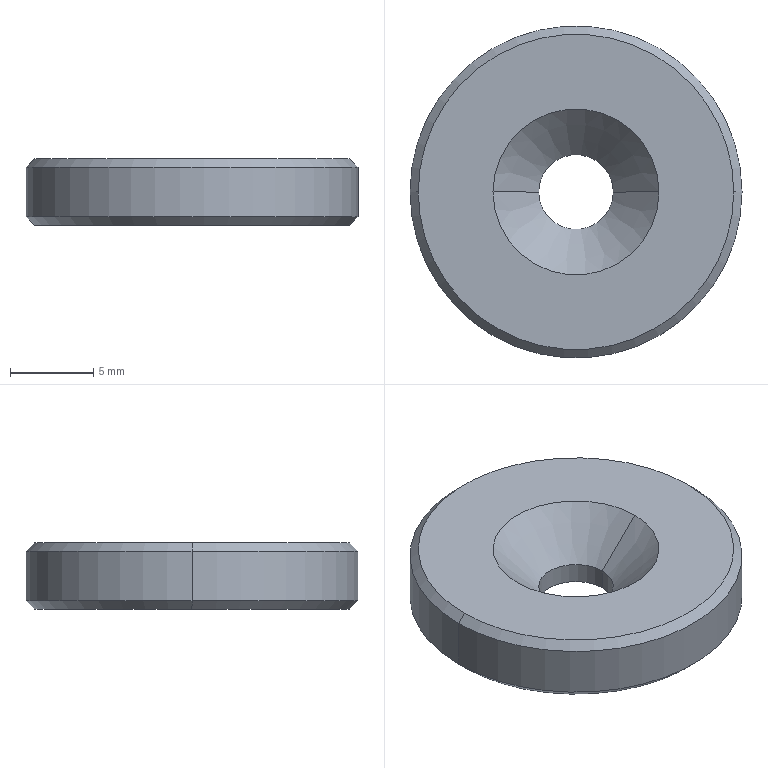Part | STEP file | 10000020547swp000-1 | 1 solid | 12 faces | box 20 x 20 x 4 mm | volume 1102 mm3 | cone 6 | cylinder 4 | plane 2 | commonest cylinder face diameters 4.5 x2 20 x2
STEP:
#1=CARTESIAN_POINT('',(9.5,0.,4.));
#2=VERTEX_POINT('',#1);
#3=CARTESIAN_POINT('',(-9.5,0.,4.));
#4=VERTEX_POINT('',#3);
#5=CARTESIAN_POINT('',(0.,0.,4.));
#6=DIRECTION('',(0.,0.,1.));
#7=DIRECTION('',(1.,0.,0.));
#8=AXIS2_PLACEMENT_3D('',#5,#6,#7);
#9=CIRCLE('',#8,9.5);
#10=EDGE_CURVE('',#2,#4,#9,.T.);
#11=ORIENTED_EDGE('',*,*,#10,.F.);
#12=CARTESIAN_POINT('',(10.,0.,3.5));
#13=VERTEX_POINT('',#12);
#14=CARTESIAN_POINT('',(9.5,0.,4.));
#15=DIRECTION('',(0.7071,0.,-0.7071));
#16=VECTOR('',#15,1000.);
#17=LINE('',#14,#16);
#18=EDGE_CURVE('',#2,#13,#17,.T.);
#19=ORIENTED_EDGE('',*,*,#18,.T.);
#20=CARTESIAN_POINT('',(-10.,0.,3.5));
#21=VERTEX_POINT('',#20);
#22=CARTESIAN_POINT('',(0.,0.,3.5));
#23=DIRECTION('',(0.,0.,-1.));
#24=DIRECTION('',(1.,0.,0.));
#25=AXIS2_PLACEMENT_3D('',#22,#23,#24);
#26=CIRCLE('',#25,10.);
#27=EDGE_CURVE('',#21,#13,#26,.T.);
#28=ORIENTED_EDGE('',*,*,#27,.F.);
#29=CARTESIAN_POINT('',(-9.5,0.,4.));
#30=DIRECTION('',(-0.7071,0.,-0.7071));
#31=VECTOR('',#30,1000.);
#32=LINE('',#29,#31);
#33=EDGE_CURVE('',#4,#21,#32,.T.);
#34=ORIENTED_EDGE('',*,*,#33,.F.);
#35=EDGE_LOOP('',(#11,#19,#28,#34));
#36=FACE_OUTER_BOUND('',#35,.T.);
#37=CARTESIAN_POINT('',(0.,0.,4.));
#38=DIRECTION('',(0.,0.,-1.));
#39=DIRECTION('',(-1.,0.,0.));
#40=AXIS2_PLACEMENT_3D('',#37,#38,#39);
#41=CONICAL_SURFACE('',#40,9.5,0.7854);
#42=ADVANCED_FACE('',(#36),#41,.T.);
#43=CARTESIAN_POINT('',(-9.5,0.,0.));
#44=VERTEX_POINT('',#43);
#45=CARTESIAN_POINT('',(9.5,0.,0.));
#46=VERTEX_POINT('',#45);
#47=CARTESIAN_POINT('',(0.,0.,0.));
#48=DIRECTION('',(0.,0.,-1.));
#49=DIRECTION('',(1.,0.,0.));
#50=AXIS2_PLACEMENT_3D('',#47,#48,#49);
#51=CIRCLE('',#50,9.5);
#52=EDGE_CURVE('',#44,#46,#51,.T.);
#53=ORIENTED_EDGE('',*,*,#52,.F.);
#54=CARTESIAN_POINT('',(-10.,0.,0.5));
#55=VERTEX_POINT('',#54);
#56=CARTESIAN_POINT('',(-10.,0.,0.5));
#57=DIRECTION('',(-0.7071,0.,0.7071));
#58=VECTOR('',#57,1000.);
#59=LINE('',#56,#58);
#60=EDGE_CURVE('',#44,#55,#59,.T.);
#61=ORIENTED_EDGE('',*,*,#60,.T.);
#62=CARTESIAN_POINT('',(10.,0.,0.5));
#63=VERTEX_POINT('',#62);
#64=CARTESIAN_POINT('',(0.,0.,0.5));
#65=DIRECTION('',(0.,0.,1.));
#66=DIRECTION('',(1.,0.,0.));
#67=AXIS2_PLACEMENT_3D('',#64,#65,#66);
#68=CIRCLE('',#67,10.);
#69=EDGE_CURVE('',#63,#55,#68,.T.);
#70=ORIENTED_EDGE('',*,*,#69,.F.);
#71=CARTESIAN_POINT('',(10.,0.,0.5));
#72=DIRECTION('',(0.7071,0.,0.7071));
#73=VECTOR('',#72,1000.);
#74=LINE('',#71,#73);
#75=EDGE_CURVE('',#46,#63,#74,.T.);
#76=ORIENTED_EDGE('',*,*,#75,.F.);
#77=EDGE_LOOP('',(#53,#61,#70,#76));
#78=FACE_OUTER_BOUND('',#77,.T.);
#79=CARTESIAN_POINT('',(0.,0.,0.5));
#80=DIRECTION('',(0.,0.,1.));
#81=DIRECTION('',(1.,0.,0.));
#82=AXIS2_PLACEMENT_3D('',#79,#80,#81);
#83=CONICAL_SURFACE('',#82,10.,0.7854);
#84=ADVANCED_FACE('',(#78),#83,.T.);
#85=CARTESIAN_POINT('',(-2.25,0.,1.25));
#86=VERTEX_POINT('',#85);
#87=CARTESIAN_POINT('',(2.25,0.,1.25));
#88=VERTEX_POINT('',#87);
#89=CARTESIAN_POINT('',(0.,0.,1.25));
#90=DIRECTION('',(0.,0.,1.));
#91=DIRECTION('',(1.,0.,0.));
#92=AXIS2_PLACEMENT_3D('',#89,#90,#91);
#93=CIRCLE('',#92,2.25);
#94=EDGE_CURVE('',#86,#88,#93,.T.);
#95=ORIENTED_EDGE('',*,*,#94,.F.);
#96=CARTESIAN_POINT('',(-5.,0.,4.));
#97=VERTEX_POINT('',#96);
#98=CARTESIAN_POINT('',(-5.,0.,4.));
#99=DIRECTION('',(-0.7071,0.,0.7071));
#100=VECTOR('',#99,1000.);
#101=LINE('',#98,#100);
#102=EDGE_CURVE('',#86,#97,#101,.T.);
#103=ORIENTED_EDGE('',*,*,#102,.T.);
#104=CARTESIAN_POINT('',(5.,0.,4.));
#105=VERTEX_POINT('',#104);
#106=CARTESIAN_POINT('',(0.,0.,4.));
#107=DIRECTION('',(0.,0.,1.));
#108=DIRECTION('',(1.,0.,0.));
#109=AXIS2_PLACEMENT_3D('',#106,#107,#108);
#110=CIRCLE('',#109,5.);
#111=EDGE_CURVE('',#97,#105,#110,.T.);
#112=ORIENTED_EDGE('',*,*,#111,.T.);
#113=CARTESIAN_POINT('',(5.,0.,4.));
#114=DIRECTION('',(0.7071,0.,0.7071));
#115=VECTOR('',#114,1000.);
#116=LINE('',#113,#115);
#117=EDGE_CURVE('',#88,#105,#116,.T.);
#118=ORIENTED_EDGE('',*,*,#117,.F.);
#119=EDGE_LOOP('',(#95,#103,#112,#118));
#120=FACE_OUTER_BOUND('',#119,.T.);
#121=CARTESIAN_POINT('',(0.,0.,4.));
#122=DIRECTION('',(0.,0.,1.));
#123=DIRECTION('',(1.,0.,0.));
#124=AXIS2_PLACEMENT_3D('',#121,#122,#123);
#125=CONICAL_SURFACE('',#124,5.,0.7854);
#126=ADVANCED_FACE('',(#120),#125,.F.);
#127=CARTESIAN_POINT('',(-2.25,0.,0.));
#128=VERTEX_POINT('',#127);
#129=CARTESIAN_POINT('',(2.25,0.,0.));
#130=VERTEX_POINT('',#129);
#131=CARTESIAN_POINT('',(0.,0.,0.));
#132=DIRECTION('',(0.,0.,1.));
#133=DIRECTION('',(1.,0.,0.));
#134=AXIS2_PLACEMENT_3D('',#131,#132,#133);
#135=CIRCLE('',#134,2.25);
#136=EDGE_CURVE('',#128,#130,#135,.T.);
#137=ORIENTED_EDGE('',*,*,#136,.F.);
#138=CARTESIAN_POINT('',(-2.25,0.,4.));
#139=DIRECTION('',(0.,0.,1.));
#140=VECTOR('',#139,1000.);
#141=LINE('',#138,#140);
#142=EDGE_CURVE('',#128,#86,#141,.T.);
#143=ORIENTED_EDGE('',*,*,#142,.T.);
#144=ORIENTED_EDGE('',*,*,#94,.T.);
#145=CARTESIAN_POINT('',(2.25,0.,4.));
#146=DIRECTION('',(0.,0.,1.));
#147=VECTOR('',#146,1000.);
#148=LINE('',#145,#147);
#149=EDGE_CURVE('',#130,#88,#148,.T.);
#150=ORIENTED_EDGE('',*,*,#149,.F.);
#151=EDGE_LOOP('',(#137,#143,#144,#150));
#152=FACE_OUTER_BOUND('',#151,.T.);
#153=CARTESIAN_POINT('',(0.,0.,4.));
#154=DIRECTION('',(0.,0.,1.));
#155=DIRECTION('',(1.,0.,0.));
#156=AXIS2_PLACEMENT_3D('',#153,#154,#155);
#157=CYLINDRICAL_SURFACE('',#156,2.25);
#158=ADVANCED_FACE('',(#152),#157,.F.);
#159=ORIENTED_EDGE('',*,*,#27,.T.);
#160=CARTESIAN_POINT('',(10.,0.,4.));
#161=DIRECTION('',(0.,0.,-1.));
#162=VECTOR('',#161,1000.);
#163=LINE('',#160,#162);
#164=EDGE_CURVE('',#13,#63,#163,.T.);
#165=ORIENTED_EDGE('',*,*,#164,.T.);
#166=ORIENTED_EDGE('',*,*,#69,.T.);
#167=CARTESIAN_POINT('',(-10.,0.,4.));
#168=DIRECTION('',(0.,0.,-1.));
#169=VECTOR('',#168,1000.);
#170=LINE('',#167,#169);
#171=EDGE_CURVE('',#21,#55,#170,.T.);
#172=ORIENTED_EDGE('',*,*,#171,.F.);
#173=EDGE_LOOP('',(#159,#165,#166,#172));
#174=FACE_OUTER_BOUND('',#173,.T.);
#175=CARTESIAN_POINT('',(0.,0.,4.));
#176=DIRECTION('',(0.,0.,-1.));
#177=DIRECTION('',(-1.,0.,0.));
#178=AXIS2_PLACEMENT_3D('',#175,#176,#177);
#179=CYLINDRICAL_SURFACE('',#178,10.);
#180=ADVANCED_FACE('',(#174),#179,.T.);
#181=ORIENTED_EDGE('',*,*,#164,.F.);
#182=CARTESIAN_POINT('',(0.,0.,3.5));
#183=DIRECTION('',(0.,0.,-1.));
#184=DIRECTION('',(1.,0.,0.));
#185=AXIS2_PLACEMENT_3D('',#182,#183,#184);
#186=CIRCLE('',#185,10.);
#187=EDGE_CURVE('',#13,#21,#186,.T.);
#188=ORIENTED_EDGE('',*,*,#187,.T.);
#189=ORIENTED_EDGE('',*,*,#171,.T.);
#190=CARTESIAN_POINT('',(0.,0.,0.5));
#191=DIRECTION('',(0.,0.,1.));
#192=DIRECTION('',(1.,0.,0.));
#193=AXIS2_PLACEMENT_3D('',#190,#191,#192);
#194=CIRCLE('',#193,10.);
#195=EDGE_CURVE('',#55,#63,#194,.T.);
#196=ORIENTED_EDGE('',*,*,#195,.T.);
#197=EDGE_LOOP('',(#181,#188,#189,#196));
#198=FACE_OUTER_BOUND('',#197,.T.);
#199=CARTESIAN_POINT('',(0.,0.,4.));
#200=DIRECTION('',(0.,0.,-1.));
#201=DIRECTION('',(-1.,0.,0.));
#202=AXIS2_PLACEMENT_3D('',#199,#200,#201);
#203=CYLINDRICAL_SURFACE('',#202,10.);
#204=ADVANCED_FACE('',(#198),#203,.T.);
#205=CARTESIAN_POINT('',(0.,0.,4.));
#206=DIRECTION('',(0.,0.,1.));
#207=DIRECTION('',(1.,0.,0.));
#208=AXIS2_PLACEMENT_3D('',#205,#206,#207);
#209=CIRCLE('',#208,9.5);
#210=EDGE_CURVE('',#4,#2,#209,.T.);
#211=ORIENTED_EDGE('',*,*,#210,.T.);
#212=ORIENTED_EDGE('',*,*,#10,.T.);
#213=EDGE_LOOP('',(#211,#212));
#214=FACE_OUTER_BOUND('',#213,.T.);
#215=CARTESIAN_POINT('',(0.,0.,4.));
#216=DIRECTION('',(0.,0.,1.));
#217=DIRECTION('',(1.,0.,0.));
#218=AXIS2_PLACEMENT_3D('',#215,#216,#217);
#219=CIRCLE('',#218,5.);
#220=EDGE_CURVE('',#105,#97,#219,.T.);
#221=ORIENTED_EDGE('',*,*,#220,.F.);
#222=ORIENTED_EDGE('',*,*,#111,.F.);
#223=EDGE_LOOP('',(#221,#222));
#224=FACE_BOUND('',#223,.T.);
#225=CARTESIAN_POINT('',(0.,0.,4.));
#226=DIRECTION('',(0.,0.,1.));
#227=DIRECTION('',(1.,0.,0.));
#228=AXIS2_PLACEMENT_3D('',#225,#226,#227);
#229=PLANE('',#228);
#230=ADVANCED_FACE('',(#214,#224),#229,.T.);
#231=CARTESIAN_POINT('',(0.,0.,0.));
#232=DIRECTION('',(0.,0.,-1.));
#233=DIRECTION('',(1.,0.,0.));
#234=AXIS2_PLACEMENT_3D('',#231,#232,#233);
#235=CIRCLE('',#234,9.5);
#236=EDGE_CURVE('',#46,#44,#235,.T.);
#237=ORIENTED_EDGE('',*,*,#236,.T.);
#238=ORIENTED_EDGE('',*,*,#52,.T.);
#239=EDGE_LOOP('',(#237,#238));
#240=FACE_OUTER_BOUND('',#239,.T.);
#241=CARTESIAN_POINT('',(0.,0.,0.));
#242=DIRECTION('',(0.,0.,1.));
#243=DIRECTION('',(1.,0.,0.));
#244=AXIS2_PLACEMENT_3D('',#241,#242,#243);
#245=CIRCLE('',#244,2.25);
#246=EDGE_CURVE('',#130,#128,#245,.T.);
#247=ORIENTED_EDGE('',*,*,#246,.T.);
#248=ORIENTED_EDGE('',*,*,#136,.T.);
#249=EDGE_LOOP('',(#247,#248));
#250=FACE_BOUND('',#249,.T.);
#251=CARTESIAN_POINT('',(0.,0.,0.));
#252=DIRECTION('',(0.,0.,1.));
#253=DIRECTION('',(1.,0.,0.));
#254=AXIS2_PLACEMENT_3D('',#251,#252,#253);
#255=PLANE('',#254);
#256=ADVANCED_FACE('',(#240,#250),#255,.F.);
#257=ORIENTED_EDGE('',*,*,#142,.F.);
#258=ORIENTED_EDGE('',*,*,#246,.F.);
#259=ORIENTED_EDGE('',*,*,#149,.T.);
#260=CARTESIAN_POINT('',(0.,0.,1.25));
#261=DIRECTION('',(0.,0.,1.));
#262=DIRECTION('',(1.,0.,0.));
#263=AXIS2_PLACEMENT_3D('',#260,#261,#262);
#264=CIRCLE('',#263,2.25);
#265=EDGE_CURVE('',#88,#86,#264,.T.);
#266=ORIENTED_EDGE('',*,*,#265,.T.);
#267=EDGE_LOOP('',(#257,#258,#259,#266));
#268=FACE_OUTER_BOUND('',#267,.T.);
#269=CARTESIAN_POINT('',(0.,0.,4.));
#270=DIRECTION('',(0.,0.,1.));
#271=DIRECTION('',(1.,0.,0.));
#272=AXIS2_PLACEMENT_3D('',#269,#270,#271);
#273=CYLINDRICAL_SURFACE('',#272,2.25);
#274=ADVANCED_FACE('',(#268),#273,.F.);
#275=ORIENTED_EDGE('',*,*,#102,.F.);
#276=ORIENTED_EDGE('',*,*,#265,.F.);
#277=ORIENTED_EDGE('',*,*,#117,.T.);
#278=ORIENTED_EDGE('',*,*,#220,.T.);
#279=EDGE_LOOP('',(#275,#276,#277,#278));
#280=FACE_OUTER_BOUND('',#279,.T.);
#281=CARTESIAN_POINT('',(0.,0.,4.));
#282=DIRECTION('',(0.,0.,1.));
#283=DIRECTION('',(1.,0.,0.));
#284=AXIS2_PLACEMENT_3D('',#281,#282,#283);
#285=CONICAL_SURFACE('',#284,5.,0.7854);
#286=ADVANCED_FACE('',(#280),#285,.F.);
#287=ORIENTED_EDGE('',*,*,#60,.F.);
#288=ORIENTED_EDGE('',*,*,#236,.F.);
#289=ORIENTED_EDGE('',*,*,#75,.T.);
#290=ORIENTED_EDGE('',*,*,#195,.F.);
#291=EDGE_LOOP('',(#287,#288,#289,#290));
#292=FACE_OUTER_BOUND('',#291,.T.);
#293=CARTESIAN_POINT('',(0.,0.,0.5));
#294=DIRECTION('',(0.,0.,1.));
#295=DIRECTION('',(1.,0.,0.));
#296=AXIS2_PLACEMENT_3D('',#293,#294,#295);
#297=CONICAL_SURFACE('',#296,10.,0.7854);
#298=ADVANCED_FACE('',(#292),#297,.T.);
#299=ORIENTED_EDGE('',*,*,#18,.F.);
#300=ORIENTED_EDGE('',*,*,#210,.F.);
#301=ORIENTED_EDGE('',*,*,#33,.T.);
#302=ORIENTED_EDGE('',*,*,#187,.F.);
#303=EDGE_LOOP('',(#299,#300,#301,#302));
#304=FACE_OUTER_BOUND('',#303,.T.);
#305=CARTESIAN_POINT('',(0.,0.,4.));
#306=DIRECTION('',(0.,0.,-1.));
#307=DIRECTION('',(-1.,0.,0.));
#308=AXIS2_PLACEMENT_3D('',#305,#306,#307);
#309=CONICAL_SURFACE('',#308,9.5,0.7854);
#310=ADVANCED_FACE('',(#304),#309,.T.);
#311=CLOSED_SHELL('',(#42,#84,#126,#158,#180,#204,#230,#256,#274,#286,#298,#310));
#312=MANIFOLD_SOLID_BREP('',#311);
#313=CARTESIAN_POINT('',(0.,0.,0.));
#314=DIRECTION('',(0.,0.,1.));
#315=DIRECTION('',(1.,0.,0.));
#316=AXIS2_PLACEMENT_3D('',#313,#314,#315);
#317=(LENGTH_UNIT()NAMED_UNIT(*)SI_UNIT(.MILLI.,.METRE.));
#318=UNCERTAINTY_MEASURE_WITH_UNIT(LENGTH_MEASURE(0.00001),#317,'','');
#319=(NAMED_UNIT(*)PLANE_ANGLE_UNIT()SI_UNIT($,.RADIAN.));
#320=(NAMED_UNIT(*)SI_UNIT($,.STERADIAN.)SOLID_ANGLE_UNIT());
#321=(GEOMETRIC_REPRESENTATION_CONTEXT(3)GLOBAL_UNCERTAINTY_ASSIGNED_CONTEXT((#318))GLOBAL_UNIT_ASSIGNED_CONTEXT((#317,#319,#320))REPRESENTATION_CONTEXT('',''));
#322=ADVANCED_BREP_SHAPE_REPRESENTATION('',(#312,#316),#321);